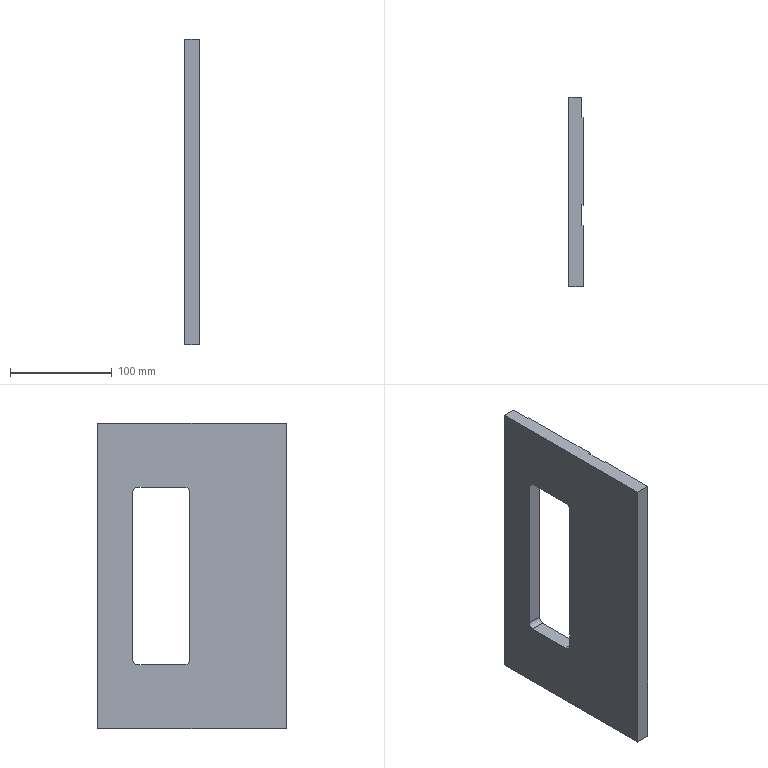Part | SolidWorks | features ICE 3, Extrusion 1, Fillet 1 | 1 solid | 20 faces | box 14 x 185 x 300 mm | volume 622434 mm3 | plane 16 | cylinder 4 | commonest cylinder face diameters 10 x4
STEP:
#1=CARTESIAN_POINT('',(14.,150.5,-82.));
#2=VERTEX_POINT('',#1);
#3=CARTESIAN_POINT('',(14.,150.5,82.));
#4=VERTEX_POINT('',#3);
#5=CARTESIAN_POINT('',(14.,150.5,87.));
#6=DIRECTION('',(0.,0.,1.));
#7=VECTOR('',#6,1000.);
#8=LINE('',#5,#7);
#9=EDGE_CURVE('',#2,#4,#8,.T.);
#10=ORIENTED_EDGE('',*,*,#9,.F.);
#11=CARTESIAN_POINT('',(14.,145.5,-87.));
#12=VERTEX_POINT('',#11);
#13=CARTESIAN_POINT('',(14.,145.5,-82.));
#14=DIRECTION('',(-1.,0.,0.));
#15=DIRECTION('',(0.,-1.,0.));
#16=AXIS2_PLACEMENT_3D('',#13,#14,#15);
#17=CIRCLE('',#16,5.);
#18=EDGE_CURVE('',#2,#12,#17,.T.);
#19=ORIENTED_EDGE('',*,*,#18,.T.);
#20=CARTESIAN_POINT('',(14.,99.5,-87.));
#21=VERTEX_POINT('',#20);
#22=CARTESIAN_POINT('',(14.,94.5,-87.));
#23=DIRECTION('',(0.,1.,0.));
#24=VECTOR('',#23,1000.);
#25=LINE('',#22,#24);
#26=EDGE_CURVE('',#21,#12,#25,.T.);
#27=ORIENTED_EDGE('',*,*,#26,.F.);
#28=CARTESIAN_POINT('',(14.,94.5,-82.));
#29=VERTEX_POINT('',#28);
#30=CARTESIAN_POINT('',(14.,99.5,-82.));
#31=DIRECTION('',(-1.,0.,0.));
#32=DIRECTION('',(0.,-1.,0.));
#33=AXIS2_PLACEMENT_3D('',#30,#31,#32);
#34=CIRCLE('',#33,5.);
#35=EDGE_CURVE('',#21,#29,#34,.T.);
#36=ORIENTED_EDGE('',*,*,#35,.T.);
#37=CARTESIAN_POINT('',(14.,94.5,82.));
#38=VERTEX_POINT('',#37);
#39=CARTESIAN_POINT('',(14.,94.5,87.));
#40=DIRECTION('',(0.,0.,-1.));
#41=VECTOR('',#40,1000.);
#42=LINE('',#39,#41);
#43=EDGE_CURVE('',#38,#29,#42,.T.);
#44=ORIENTED_EDGE('',*,*,#43,.F.);
#45=CARTESIAN_POINT('',(14.,99.5,87.));
#46=VERTEX_POINT('',#45);
#47=CARTESIAN_POINT('',(14.,99.5,82.));
#48=DIRECTION('',(-1.,0.,0.));
#49=DIRECTION('',(0.,-1.,0.));
#50=AXIS2_PLACEMENT_3D('',#47,#48,#49);
#51=CIRCLE('',#50,5.);
#52=EDGE_CURVE('',#38,#46,#51,.T.);
#53=ORIENTED_EDGE('',*,*,#52,.T.);
#54=CARTESIAN_POINT('',(14.,145.5,87.));
#55=VERTEX_POINT('',#54);
#56=CARTESIAN_POINT('',(14.,94.5,87.));
#57=DIRECTION('',(0.,-1.,0.));
#58=VECTOR('',#57,1000.);
#59=LINE('',#56,#58);
#60=EDGE_CURVE('',#55,#46,#59,.T.);
#61=ORIENTED_EDGE('',*,*,#60,.F.);
#62=CARTESIAN_POINT('',(14.,145.5,82.));
#63=DIRECTION('',(-1.,0.,0.));
#64=DIRECTION('',(0.,-1.,0.));
#65=AXIS2_PLACEMENT_3D('',#62,#63,#64);
#66=CIRCLE('',#65,5.);
#67=EDGE_CURVE('',#55,#4,#66,.T.);
#68=ORIENTED_EDGE('',*,*,#67,.T.);
#69=EDGE_LOOP('',(#10,#19,#27,#36,#44,#53,#61,#68));
#70=FACE_BOUND('',#69,.T.);
#71=CARTESIAN_POINT('',(14.,80.,-150.));
#72=VERTEX_POINT('',#71);
#73=CARTESIAN_POINT('',(14.,165.,-150.));
#74=VERTEX_POINT('',#73);
#75=CARTESIAN_POINT('',(14.,185.,-150.));
#76=DIRECTION('',(0.,1.,0.));
#77=VECTOR('',#76,1000.);
#78=LINE('',#75,#77);
#79=EDGE_CURVE('',#72,#74,#78,.T.);
#80=ORIENTED_EDGE('',*,*,#79,.T.);
#81=CARTESIAN_POINT('',(14.,165.,150.));
#82=VERTEX_POINT('',#81);
#83=CARTESIAN_POINT('',(14.,165.,150.));
#84=DIRECTION('',(0.,0.,-1.));
#85=VECTOR('',#84,1000.);
#86=LINE('',#83,#85);
#87=EDGE_CURVE('',#82,#74,#86,.T.);
#88=ORIENTED_EDGE('',*,*,#87,.F.);
#89=CARTESIAN_POINT('',(14.,80.,150.));
#90=VERTEX_POINT('',#89);
#91=CARTESIAN_POINT('',(14.,185.,150.));
#92=DIRECTION('',(0.,1.,0.));
#93=VECTOR('',#92,1000.);
#94=LINE('',#91,#93);
#95=EDGE_CURVE('',#90,#82,#94,.T.);
#96=ORIENTED_EDGE('',*,*,#95,.F.);
#97=CARTESIAN_POINT('',(14.,80.,150.));
#98=DIRECTION('',(0.,0.,1.));
#99=VECTOR('',#98,1000.);
#100=LINE('',#97,#99);
#101=EDGE_CURVE('',#72,#90,#100,.T.);
#102=ORIENTED_EDGE('',*,*,#101,.F.);
#103=EDGE_LOOP('',(#80,#88,#96,#102));
#104=FACE_OUTER_BOUND('',#103,.T.);
#105=CARTESIAN_POINT('',(14.,185.,150.));
#106=DIRECTION('',(-1.,0.,0.));
#107=DIRECTION('',(0.,-1.,0.));
#108=AXIS2_PLACEMENT_3D('',#105,#106,#107);
#109=PLANE('',#108);
#110=ADVANCED_FACE('',(#70,#104),#109,.F.);
#111=CARTESIAN_POINT('',(12.5,185.,-150.));
#112=VERTEX_POINT('',#111);
#113=CARTESIAN_POINT('',(12.5,185.,150.));
#114=VERTEX_POINT('',#113);
#115=CARTESIAN_POINT('',(12.5,185.,150.));
#116=DIRECTION('',(0.,0.,1.));
#117=VECTOR('',#116,1000.);
#118=LINE('',#115,#117);
#119=EDGE_CURVE('',#112,#114,#118,.T.);
#120=ORIENTED_EDGE('',*,*,#119,.F.);
#121=CARTESIAN_POINT('',(0.,185.,-150.));
#122=VERTEX_POINT('',#121);
#123=CARTESIAN_POINT('',(0.,185.,-150.));
#124=DIRECTION('',(-1.,0.,0.));
#125=VECTOR('',#124,1000.);
#126=LINE('',#123,#125);
#127=EDGE_CURVE('',#112,#122,#126,.T.);
#128=ORIENTED_EDGE('',*,*,#127,.T.);
#129=CARTESIAN_POINT('',(0.,185.,150.));
#130=VERTEX_POINT('',#129);
#131=CARTESIAN_POINT('',(0.,185.,150.));
#132=DIRECTION('',(0.,0.,-1.));
#133=VECTOR('',#132,1000.);
#134=LINE('',#131,#133);
#135=EDGE_CURVE('',#130,#122,#134,.T.);
#136=ORIENTED_EDGE('',*,*,#135,.F.);
#137=CARTESIAN_POINT('',(0.,185.,150.));
#138=DIRECTION('',(-1.,0.,0.));
#139=VECTOR('',#138,1000.);
#140=LINE('',#137,#139);
#141=EDGE_CURVE('',#114,#130,#140,.T.);
#142=ORIENTED_EDGE('',*,*,#141,.F.);
#143=EDGE_LOOP('',(#120,#128,#136,#142));
#144=FACE_OUTER_BOUND('',#143,.T.);
#145=CARTESIAN_POINT('',(0.,185.,150.));
#146=DIRECTION('',(0.,-1.,0.));
#147=DIRECTION('',(0.,0.,-1.));
#148=AXIS2_PLACEMENT_3D('',#145,#146,#147);
#149=PLANE('',#148);
#150=ADVANCED_FACE('',(#144),#149,.F.);
#151=CARTESIAN_POINT('',(0.,0.,-150.));
#152=VERTEX_POINT('',#151);
#153=CARTESIAN_POINT('',(14.,0.,-150.));
#154=VERTEX_POINT('',#153);
#155=CARTESIAN_POINT('',(0.,0.,-150.));
#156=DIRECTION('',(1.,0.,0.));
#157=VECTOR('',#156,1000.);
#158=LINE('',#155,#157);
#159=EDGE_CURVE('',#152,#154,#158,.T.);
#160=ORIENTED_EDGE('',*,*,#159,.T.);
#161=CARTESIAN_POINT('',(14.,0.,150.));
#162=VERTEX_POINT('',#161);
#163=CARTESIAN_POINT('',(14.,0.,150.));
#164=DIRECTION('',(0.,0.,-1.));
#165=VECTOR('',#164,1000.);
#166=LINE('',#163,#165);
#167=EDGE_CURVE('',#162,#154,#166,.T.);
#168=ORIENTED_EDGE('',*,*,#167,.F.);
#169=CARTESIAN_POINT('',(0.,0.,150.));
#170=VERTEX_POINT('',#169);
#171=CARTESIAN_POINT('',(0.,0.,150.));
#172=DIRECTION('',(1.,0.,0.));
#173=VECTOR('',#172,1000.);
#174=LINE('',#171,#173);
#175=EDGE_CURVE('',#170,#162,#174,.T.);
#176=ORIENTED_EDGE('',*,*,#175,.F.);
#177=CARTESIAN_POINT('',(0.,0.,150.));
#178=DIRECTION('',(0.,0.,-1.));
#179=VECTOR('',#178,1000.);
#180=LINE('',#177,#179);
#181=EDGE_CURVE('',#170,#152,#180,.T.);
#182=ORIENTED_EDGE('',*,*,#181,.T.);
#183=EDGE_LOOP('',(#160,#168,#176,#182));
#184=FACE_OUTER_BOUND('',#183,.T.);
#185=CARTESIAN_POINT('',(0.,0.,150.));
#186=DIRECTION('',(0.,1.,0.));
#187=DIRECTION('',(0.,0.,1.));
#188=AXIS2_PLACEMENT_3D('',#185,#186,#187);
#189=PLANE('',#188);
#190=ADVANCED_FACE('',(#184),#189,.F.);
#191=CARTESIAN_POINT('',(14.,59.,-150.));
#192=VERTEX_POINT('',#191);
#193=CARTESIAN_POINT('',(14.,185.,-150.));
#194=DIRECTION('',(0.,1.,0.));
#195=VECTOR('',#194,1000.);
#196=LINE('',#193,#195);
#197=EDGE_CURVE('',#154,#192,#196,.T.);
#198=ORIENTED_EDGE('',*,*,#197,.T.);
#199=CARTESIAN_POINT('',(14.,59.,150.));
#200=VERTEX_POINT('',#199);
#201=CARTESIAN_POINT('',(14.,59.,150.));
#202=DIRECTION('',(0.,0.,-1.));
#203=VECTOR('',#202,1000.);
#204=LINE('',#201,#203);
#205=EDGE_CURVE('',#200,#192,#204,.T.);
#206=ORIENTED_EDGE('',*,*,#205,.F.);
#207=CARTESIAN_POINT('',(14.,185.,150.));
#208=DIRECTION('',(0.,1.,0.));
#209=VECTOR('',#208,1000.);
#210=LINE('',#207,#209);
#211=EDGE_CURVE('',#162,#200,#210,.T.);
#212=ORIENTED_EDGE('',*,*,#211,.F.);
#213=ORIENTED_EDGE('',*,*,#167,.T.);
#214=EDGE_LOOP('',(#198,#206,#212,#213));
#215=FACE_OUTER_BOUND('',#214,.T.);
#216=CARTESIAN_POINT('',(14.,185.,150.));
#217=DIRECTION('',(-1.,0.,0.));
#218=DIRECTION('',(0.,-1.,0.));
#219=AXIS2_PLACEMENT_3D('',#216,#217,#218);
#220=PLANE('',#219);
#221=ADVANCED_FACE('',(#215),#220,.F.);
#222=CARTESIAN_POINT('',(0.,94.5,-82.));
#223=VERTEX_POINT('',#222);
#224=CARTESIAN_POINT('',(0.,94.5,82.));
#225=VERTEX_POINT('',#224);
#226=CARTESIAN_POINT('',(0.,94.5,87.));
#227=DIRECTION('',(0.,0.,1.));
#228=VECTOR('',#227,1000.);
#229=LINE('',#226,#228);
#230=EDGE_CURVE('',#223,#225,#229,.T.);
#231=ORIENTED_EDGE('',*,*,#230,.F.);
#232=CARTESIAN_POINT('',(0.,99.5,-87.));
#233=VERTEX_POINT('',#232);
#234=CARTESIAN_POINT('',(0.,99.5,-82.));
#235=DIRECTION('',(1.,0.,0.));
#236=DIRECTION('',(0.,1.,0.));
#237=AXIS2_PLACEMENT_3D('',#234,#235,#236);
#238=CIRCLE('',#237,5.);
#239=EDGE_CURVE('',#223,#233,#238,.T.);
#240=ORIENTED_EDGE('',*,*,#239,.T.);
#241=CARTESIAN_POINT('',(0.,145.5,-87.));
#242=VERTEX_POINT('',#241);
#243=CARTESIAN_POINT('',(0.,94.5,-87.));
#244=DIRECTION('',(0.,-1.,0.));
#245=VECTOR('',#244,1000.);
#246=LINE('',#243,#245);
#247=EDGE_CURVE('',#242,#233,#246,.T.);
#248=ORIENTED_EDGE('',*,*,#247,.F.);
#249=CARTESIAN_POINT('',(0.,150.5,-82.));
#250=VERTEX_POINT('',#249);
#251=CARTESIAN_POINT('',(0.,145.5,-82.));
#252=DIRECTION('',(1.,0.,0.));
#253=DIRECTION('',(0.,1.,0.));
#254=AXIS2_PLACEMENT_3D('',#251,#252,#253);
#255=CIRCLE('',#254,5.);
#256=EDGE_CURVE('',#242,#250,#255,.T.);
#257=ORIENTED_EDGE('',*,*,#256,.T.);
#258=CARTESIAN_POINT('',(0.,150.5,82.));
#259=VERTEX_POINT('',#258);
#260=CARTESIAN_POINT('',(0.,150.5,87.));
#261=DIRECTION('',(0.,0.,-1.));
#262=VECTOR('',#261,1000.);
#263=LINE('',#260,#262);
#264=EDGE_CURVE('',#259,#250,#263,.T.);
#265=ORIENTED_EDGE('',*,*,#264,.F.);
#266=CARTESIAN_POINT('',(0.,145.5,87.));
#267=VERTEX_POINT('',#266);
#268=CARTESIAN_POINT('',(0.,145.5,82.));
#269=DIRECTION('',(1.,0.,0.));
#270=DIRECTION('',(0.,1.,0.));
#271=AXIS2_PLACEMENT_3D('',#268,#269,#270);
#272=CIRCLE('',#271,5.);
#273=EDGE_CURVE('',#259,#267,#272,.T.);
#274=ORIENTED_EDGE('',*,*,#273,.T.);
#275=CARTESIAN_POINT('',(0.,99.5,87.));
#276=VERTEX_POINT('',#275);
#277=CARTESIAN_POINT('',(0.,94.5,87.));
#278=DIRECTION('',(0.,1.,0.));
#279=VECTOR('',#278,1000.);
#280=LINE('',#277,#279);
#281=EDGE_CURVE('',#276,#267,#280,.T.);
#282=ORIENTED_EDGE('',*,*,#281,.F.);
#283=CARTESIAN_POINT('',(0.,99.5,82.));
#284=DIRECTION('',(1.,0.,0.));
#285=DIRECTION('',(0.,1.,0.));
#286=AXIS2_PLACEMENT_3D('',#283,#284,#285);
#287=CIRCLE('',#286,5.);
#288=EDGE_CURVE('',#276,#225,#287,.T.);
#289=ORIENTED_EDGE('',*,*,#288,.T.);
#290=EDGE_LOOP('',(#231,#240,#248,#257,#265,#274,#282,#289));
#291=FACE_BOUND('',#290,.T.);
#292=CARTESIAN_POINT('',(0.,0.,-150.));
#293=DIRECTION('',(0.,-1.,0.));
#294=VECTOR('',#293,1000.);
#295=LINE('',#292,#294);
#296=EDGE_CURVE('',#122,#152,#295,.T.);
#297=ORIENTED_EDGE('',*,*,#296,.T.);
#298=ORIENTED_EDGE('',*,*,#181,.F.);
#299=CARTESIAN_POINT('',(0.,0.,150.));
#300=DIRECTION('',(0.,-1.,0.));
#301=VECTOR('',#300,1000.);
#302=LINE('',#299,#301);
#303=EDGE_CURVE('',#130,#170,#302,.T.);
#304=ORIENTED_EDGE('',*,*,#303,.F.);
#305=ORIENTED_EDGE('',*,*,#135,.T.);
#306=EDGE_LOOP('',(#297,#298,#304,#305));
#307=FACE_OUTER_BOUND('',#306,.T.);
#308=CARTESIAN_POINT('',(0.,0.,150.));
#309=DIRECTION('',(1.,0.,0.));
#310=DIRECTION('',(0.,1.,0.));
#311=AXIS2_PLACEMENT_3D('',#308,#309,#310);
#312=PLANE('',#311);
#313=ADVANCED_FACE('',(#291,#307),#312,.F.);
#314=ORIENTED_EDGE('',*,*,#95,.T.);
#315=CARTESIAN_POINT('',(12.5,165.,150.));
#316=VERTEX_POINT('',#315);
#317=CARTESIAN_POINT('',(12.5,165.,150.));
#318=DIRECTION('',(1.,0.,0.));
#319=VECTOR('',#318,1000.);
#320=LINE('',#317,#319);
#321=EDGE_CURVE('',#316,#82,#320,.T.);
#322=ORIENTED_EDGE('',*,*,#321,.F.);
#323=CARTESIAN_POINT('',(12.5,185.,150.));
#324=DIRECTION('',(0.,-1.,0.));
#325=VECTOR('',#324,1000.);
#326=LINE('',#323,#325);
#327=EDGE_CURVE('',#114,#316,#326,.T.);
#328=ORIENTED_EDGE('',*,*,#327,.F.);
#329=ORIENTED_EDGE('',*,*,#141,.T.);
#330=ORIENTED_EDGE('',*,*,#303,.T.);
#331=ORIENTED_EDGE('',*,*,#175,.T.);
#332=ORIENTED_EDGE('',*,*,#211,.T.);
#333=CARTESIAN_POINT('',(12.5,59.,150.));
#334=VERTEX_POINT('',#333);
#335=CARTESIAN_POINT('',(12.5,59.,150.));
#336=DIRECTION('',(1.,0.,0.));
#337=VECTOR('',#336,1000.);
#338=LINE('',#335,#337);
#339=EDGE_CURVE('',#334,#200,#338,.T.);
#340=ORIENTED_EDGE('',*,*,#339,.F.);
#341=CARTESIAN_POINT('',(12.5,80.,150.));
#342=VERTEX_POINT('',#341);
#343=CARTESIAN_POINT('',(12.5,80.,150.));
#344=DIRECTION('',(0.,-1.,0.));
#345=VECTOR('',#344,1000.);
#346=LINE('',#343,#345);
#347=EDGE_CURVE('',#342,#334,#346,.T.);
#348=ORIENTED_EDGE('',*,*,#347,.F.);
#349=CARTESIAN_POINT('',(12.5,80.,150.));
#350=DIRECTION('',(1.,0.,0.));
#351=VECTOR('',#350,1000.);
#352=LINE('',#349,#351);
#353=EDGE_CURVE('',#342,#90,#352,.T.);
#354=ORIENTED_EDGE('',*,*,#353,.T.);
#355=EDGE_LOOP('',(#314,#322,#328,#329,#330,#331,#332,#340,#348,#354));
#356=FACE_OUTER_BOUND('',#355,.T.);
#357=CARTESIAN_POINT('',(0.,0.,150.));
#358=DIRECTION('',(0.,0.,-1.));
#359=DIRECTION('',(-1.,0.,0.));
#360=AXIS2_PLACEMENT_3D('',#357,#358,#359);
#361=PLANE('',#360);
#362=ADVANCED_FACE('',(#356),#361,.F.);
#363=CARTESIAN_POINT('',(12.5,165.,-150.));
#364=VERTEX_POINT('',#363);
#365=CARTESIAN_POINT('',(12.5,165.,-150.));
#366=DIRECTION('',(1.,0.,0.));
#367=VECTOR('',#366,1000.);
#368=LINE('',#365,#367);
#369=EDGE_CURVE('',#364,#74,#368,.T.);
#370=ORIENTED_EDGE('',*,*,#369,.T.);
#371=ORIENTED_EDGE('',*,*,#79,.F.);
#372=CARTESIAN_POINT('',(12.5,80.,-150.));
#373=VERTEX_POINT('',#372);
#374=CARTESIAN_POINT('',(12.5,80.,-150.));
#375=DIRECTION('',(1.,0.,0.));
#376=VECTOR('',#375,1000.);
#377=LINE('',#374,#376);
#378=EDGE_CURVE('',#373,#72,#377,.T.);
#379=ORIENTED_EDGE('',*,*,#378,.F.);
#380=CARTESIAN_POINT('',(12.5,59.,-150.));
#381=VERTEX_POINT('',#380);
#382=CARTESIAN_POINT('',(12.5,80.,-150.));
#383=DIRECTION('',(0.,1.,0.));
#384=VECTOR('',#383,1000.);
#385=LINE('',#382,#384);
#386=EDGE_CURVE('',#381,#373,#385,.T.);
#387=ORIENTED_EDGE('',*,*,#386,.F.);
#388=CARTESIAN_POINT('',(12.5,59.,-150.));
#389=DIRECTION('',(1.,0.,0.));
#390=VECTOR('',#389,1000.);
#391=LINE('',#388,#390);
#392=EDGE_CURVE('',#381,#192,#391,.T.);
#393=ORIENTED_EDGE('',*,*,#392,.T.);
#394=ORIENTED_EDGE('',*,*,#197,.F.);
#395=ORIENTED_EDGE('',*,*,#159,.F.);
#396=ORIENTED_EDGE('',*,*,#296,.F.);
#397=ORIENTED_EDGE('',*,*,#127,.F.);
#398=CARTESIAN_POINT('',(12.5,185.,-150.));
#399=DIRECTION('',(0.,1.,0.));
#400=VECTOR('',#399,1000.);
#401=LINE('',#398,#400);
#402=EDGE_CURVE('',#364,#112,#401,.T.);
#403=ORIENTED_EDGE('',*,*,#402,.F.);
#404=EDGE_LOOP('',(#370,#371,#379,#387,#393,#394,#395,#396,#397,#403));
#405=FACE_OUTER_BOUND('',#404,.T.);
#406=CARTESIAN_POINT('',(0.,0.,-150.));
#407=DIRECTION('',(0.,0.,-1.));
#408=DIRECTION('',(-1.,0.,0.));
#409=AXIS2_PLACEMENT_3D('',#406,#407,#408);
#410=PLANE('',#409);
#411=ADVANCED_FACE('',(#405),#410,.T.);
#412=ORIENTED_EDGE('',*,*,#101,.T.);
#413=ORIENTED_EDGE('',*,*,#353,.F.);
#414=CARTESIAN_POINT('',(12.5,80.,150.));
#415=DIRECTION('',(0.,0.,1.));
#416=VECTOR('',#415,1000.);
#417=LINE('',#414,#416);
#418=EDGE_CURVE('',#373,#342,#417,.T.);
#419=ORIENTED_EDGE('',*,*,#418,.F.);
#420=ORIENTED_EDGE('',*,*,#378,.T.);
#421=EDGE_LOOP('',(#412,#413,#419,#420));
#422=FACE_OUTER_BOUND('',#421,.T.);
#423=CARTESIAN_POINT('',(12.5,80.,150.));
#424=DIRECTION('',(0.,1.,0.));
#425=DIRECTION('',(-1.,0.,0.));
#426=AXIS2_PLACEMENT_3D('',#423,#424,#425);
#427=PLANE('',#426);
#428=ADVANCED_FACE('',(#422),#427,.F.);
#429=ORIENTED_EDGE('',*,*,#205,.T.);
#430=ORIENTED_EDGE('',*,*,#392,.F.);
#431=CARTESIAN_POINT('',(12.5,59.,150.));
#432=DIRECTION('',(0.,0.,-1.));
#433=VECTOR('',#432,1000.);
#434=LINE('',#431,#433);
#435=EDGE_CURVE('',#334,#381,#434,.T.);
#436=ORIENTED_EDGE('',*,*,#435,.F.);
#437=ORIENTED_EDGE('',*,*,#339,.T.);
#438=EDGE_LOOP('',(#429,#430,#436,#437));
#439=FACE_OUTER_BOUND('',#438,.T.);
#440=CARTESIAN_POINT('',(12.5,59.,150.));
#441=DIRECTION('',(0.,-1.,0.));
#442=DIRECTION('',(1.,0.,0.));
#443=AXIS2_PLACEMENT_3D('',#440,#441,#442);
#444=PLANE('',#443);
#445=ADVANCED_FACE('',(#439),#444,.F.);
#446=ORIENTED_EDGE('',*,*,#347,.T.);
#447=ORIENTED_EDGE('',*,*,#435,.T.);
#448=ORIENTED_EDGE('',*,*,#386,.T.);
#449=ORIENTED_EDGE('',*,*,#418,.T.);
#450=EDGE_LOOP('',(#446,#447,#448,#449));
#451=FACE_OUTER_BOUND('',#450,.T.);
#452=CARTESIAN_POINT('',(12.5,0.,0.));
#453=DIRECTION('',(1.,0.,0.));
#454=DIRECTION('',(0.,1.,0.));
#455=AXIS2_PLACEMENT_3D('',#452,#453,#454);
#456=PLANE('',#455);
#457=ADVANCED_FACE('',(#451),#456,.T.);
#458=ORIENTED_EDGE('',*,*,#87,.T.);
#459=ORIENTED_EDGE('',*,*,#369,.F.);
#460=CARTESIAN_POINT('',(12.5,165.,150.));
#461=DIRECTION('',(0.,0.,-1.));
#462=VECTOR('',#461,1000.);
#463=LINE('',#460,#462);
#464=EDGE_CURVE('',#316,#364,#463,.T.);
#465=ORIENTED_EDGE('',*,*,#464,.F.);
#466=ORIENTED_EDGE('',*,*,#321,.T.);
#467=EDGE_LOOP('',(#458,#459,#465,#466));
#468=FACE_OUTER_BOUND('',#467,.T.);
#469=CARTESIAN_POINT('',(12.5,165.,150.));
#470=DIRECTION('',(0.,-1.,0.));
#471=DIRECTION('',(1.,0.,0.));
#472=AXIS2_PLACEMENT_3D('',#469,#470,#471);
#473=PLANE('',#472);
#474=ADVANCED_FACE('',(#468),#473,.F.);
#475=ORIENTED_EDGE('',*,*,#327,.T.);
#476=ORIENTED_EDGE('',*,*,#464,.T.);
#477=ORIENTED_EDGE('',*,*,#402,.T.);
#478=ORIENTED_EDGE('',*,*,#119,.T.);
#479=EDGE_LOOP('',(#475,#476,#477,#478));
#480=FACE_OUTER_BOUND('',#479,.T.);
#481=CARTESIAN_POINT('',(12.5,0.,0.));
#482=DIRECTION('',(1.,0.,0.));
#483=DIRECTION('',(0.,1.,0.));
#484=AXIS2_PLACEMENT_3D('',#481,#482,#483);
#485=PLANE('',#484);
#486=ADVANCED_FACE('',(#480),#485,.T.);
#487=ORIENTED_EDGE('',*,*,#247,.T.);
#488=CARTESIAN_POINT('',(14.,99.5,-87.));
#489=DIRECTION('',(1.,0.,0.));
#490=VECTOR('',#489,1000.);
#491=LINE('',#488,#490);
#492=EDGE_CURVE('',#233,#21,#491,.T.);
#493=ORIENTED_EDGE('',*,*,#492,.T.);
#494=ORIENTED_EDGE('',*,*,#26,.T.);
#495=CARTESIAN_POINT('',(0.,145.5,-87.));
#496=DIRECTION('',(-1.,0.,0.));
#497=VECTOR('',#496,1000.);
#498=LINE('',#495,#497);
#499=EDGE_CURVE('',#12,#242,#498,.T.);
#500=ORIENTED_EDGE('',*,*,#499,.T.);
#501=EDGE_LOOP('',(#487,#493,#494,#500));
#502=FACE_OUTER_BOUND('',#501,.T.);
#503=CARTESIAN_POINT('',(-0.001,94.5,-87.));
#504=DIRECTION('',(0.,0.,-1.));
#505=DIRECTION('',(-1.,0.,0.));
#506=AXIS2_PLACEMENT_3D('',#503,#504,#505);
#507=PLANE('',#506);
#508=ADVANCED_FACE('',(#502),#507,.F.);
#509=ORIENTED_EDGE('',*,*,#230,.T.);
#510=CARTESIAN_POINT('',(14.,94.5,82.));
#511=DIRECTION('',(1.,0.,0.));
#512=VECTOR('',#511,1000.);
#513=LINE('',#510,#512);
#514=EDGE_CURVE('',#225,#38,#513,.T.);
#515=ORIENTED_EDGE('',*,*,#514,.T.);
#516=ORIENTED_EDGE('',*,*,#43,.T.);
#517=CARTESIAN_POINT('',(0.,94.5,-82.));
#518=DIRECTION('',(-1.,0.,0.));
#519=VECTOR('',#518,1000.);
#520=LINE('',#517,#519);
#521=EDGE_CURVE('',#29,#223,#520,.T.);
#522=ORIENTED_EDGE('',*,*,#521,.T.);
#523=EDGE_LOOP('',(#509,#515,#516,#522));
#524=FACE_OUTER_BOUND('',#523,.T.);
#525=CARTESIAN_POINT('',(-0.001,94.5,87.));
#526=DIRECTION('',(0.,-1.,0.));
#527=DIRECTION('',(1.,0.,0.));
#528=AXIS2_PLACEMENT_3D('',#525,#526,#527);
#529=PLANE('',#528);
#530=ADVANCED_FACE('',(#524),#529,.F.);
#531=ORIENTED_EDGE('',*,*,#60,.T.);
#532=CARTESIAN_POINT('',(0.,99.5,87.));
#533=DIRECTION('',(-1.,0.,0.));
#534=VECTOR('',#533,1000.);
#535=LINE('',#532,#534);
#536=EDGE_CURVE('',#46,#276,#535,.T.);
#537=ORIENTED_EDGE('',*,*,#536,.T.);
#538=ORIENTED_EDGE('',*,*,#281,.T.);
#539=CARTESIAN_POINT('',(14.,145.5,87.));
#540=DIRECTION('',(1.,0.,0.));
#541=VECTOR('',#540,1000.);
#542=LINE('',#539,#541);
#543=EDGE_CURVE('',#267,#55,#542,.T.);
#544=ORIENTED_EDGE('',*,*,#543,.T.);
#545=EDGE_LOOP('',(#531,#537,#538,#544));
#546=FACE_OUTER_BOUND('',#545,.T.);
#547=CARTESIAN_POINT('',(-0.001,94.5,87.));
#548=DIRECTION('',(0.,0.,1.));
#549=DIRECTION('',(1.,0.,0.));
#550=AXIS2_PLACEMENT_3D('',#547,#548,#549);
#551=PLANE('',#550);
#552=ADVANCED_FACE('',(#546),#551,.F.);
#553=ORIENTED_EDGE('',*,*,#9,.T.);
#554=CARTESIAN_POINT('',(0.,150.5,82.));
#555=DIRECTION('',(-1.,0.,0.));
#556=VECTOR('',#555,1000.);
#557=LINE('',#554,#556);
#558=EDGE_CURVE('',#4,#259,#557,.T.);
#559=ORIENTED_EDGE('',*,*,#558,.T.);
#560=ORIENTED_EDGE('',*,*,#264,.T.);
#561=CARTESIAN_POINT('',(14.,150.5,-82.));
#562=DIRECTION('',(1.,0.,0.));
#563=VECTOR('',#562,1000.);
#564=LINE('',#561,#563);
#565=EDGE_CURVE('',#250,#2,#564,.T.);
#566=ORIENTED_EDGE('',*,*,#565,.T.);
#567=EDGE_LOOP('',(#553,#559,#560,#566));
#568=FACE_OUTER_BOUND('',#567,.T.);
#569=CARTESIAN_POINT('',(-0.001,150.5,87.));
#570=DIRECTION('',(0.,1.,0.));
#571=DIRECTION('',(-1.,0.,0.));
#572=AXIS2_PLACEMENT_3D('',#569,#570,#571);
#573=PLANE('',#572);
#574=ADVANCED_FACE('',(#568),#573,.F.);
#575=ORIENTED_EDGE('',*,*,#288,.F.);
#576=ORIENTED_EDGE('',*,*,#536,.F.);
#577=ORIENTED_EDGE('',*,*,#52,.F.);
#578=ORIENTED_EDGE('',*,*,#514,.F.);
#579=EDGE_LOOP('',(#575,#576,#577,#578));
#580=FACE_OUTER_BOUND('',#579,.T.);
#581=CARTESIAN_POINT('',(-0.001,99.5,82.));
#582=DIRECTION('',(-1.,0.,0.));
#583=DIRECTION('',(0.,-1.,0.));
#584=AXIS2_PLACEMENT_3D('',#581,#582,#583);
#585=CYLINDRICAL_SURFACE('',#584,5.);
#586=ADVANCED_FACE('',(#580),#585,.F.);
#587=ORIENTED_EDGE('',*,*,#273,.F.);
#588=ORIENTED_EDGE('',*,*,#558,.F.);
#589=ORIENTED_EDGE('',*,*,#67,.F.);
#590=ORIENTED_EDGE('',*,*,#543,.F.);
#591=EDGE_LOOP('',(#587,#588,#589,#590));
#592=FACE_OUTER_BOUND('',#591,.T.);
#593=CARTESIAN_POINT('',(-0.001,145.5,82.));
#594=DIRECTION('',(-1.,0.,0.));
#595=DIRECTION('',(0.,-1.,0.));
#596=AXIS2_PLACEMENT_3D('',#593,#594,#595);
#597=CYLINDRICAL_SURFACE('',#596,5.);
#598=ADVANCED_FACE('',(#592),#597,.F.);
#599=ORIENTED_EDGE('',*,*,#239,.F.);
#600=ORIENTED_EDGE('',*,*,#521,.F.);
#601=ORIENTED_EDGE('',*,*,#35,.F.);
#602=ORIENTED_EDGE('',*,*,#492,.F.);
#603=EDGE_LOOP('',(#599,#600,#601,#602));
#604=FACE_OUTER_BOUND('',#603,.T.);
#605=CARTESIAN_POINT('',(-0.001,99.5,-82.));
#606=DIRECTION('',(-1.,0.,0.));
#607=DIRECTION('',(0.,-1.,0.));
#608=AXIS2_PLACEMENT_3D('',#605,#606,#607);
#609=CYLINDRICAL_SURFACE('',#608,5.);
#610=ADVANCED_FACE('',(#604),#609,.F.);
#611=ORIENTED_EDGE('',*,*,#256,.F.);
#612=ORIENTED_EDGE('',*,*,#499,.F.);
#613=ORIENTED_EDGE('',*,*,#18,.F.);
#614=ORIENTED_EDGE('',*,*,#565,.F.);
#615=EDGE_LOOP('',(#611,#612,#613,#614));
#616=FACE_OUTER_BOUND('',#615,.T.);
#617=CARTESIAN_POINT('',(-0.001,145.5,-82.));
#618=DIRECTION('',(-1.,0.,0.));
#619=DIRECTION('',(0.,-1.,0.));
#620=AXIS2_PLACEMENT_3D('',#617,#618,#619);
#621=CYLINDRICAL_SURFACE('',#620,5.);
#622=ADVANCED_FACE('',(#616),#621,.F.);
#623=CLOSED_SHELL('',(#110,#150,#190,#221,#313,#362,#411,#428,#445,#457,#474,#486,#508,#530,#552,#574,#586,#598,#610,#622));
#624=MANIFOLD_SOLID_BREP('',#623);
#625=CARTESIAN_POINT('',(0.,0.,0.));
#626=DIRECTION('',(0.,0.,1.));
#627=DIRECTION('',(1.,0.,0.));
#628=AXIS2_PLACEMENT_3D('',#625,#626,#627);
#629=(LENGTH_UNIT()NAMED_UNIT(*)SI_UNIT(.MILLI.,.METRE.));
#630=UNCERTAINTY_MEASURE_WITH_UNIT(LENGTH_MEASURE(0.00001),#629,'','');
#631=(NAMED_UNIT(*)PLANE_ANGLE_UNIT()SI_UNIT($,.RADIAN.));
#632=(NAMED_UNIT(*)SI_UNIT($,.STERADIAN.)SOLID_ANGLE_UNIT());
#633=(GEOMETRIC_REPRESENTATION_CONTEXT(3)GLOBAL_UNCERTAINTY_ASSIGNED_CONTEXT((#630))GLOBAL_UNIT_ASSIGNED_CONTEXT((#629,#631,#632))REPRESENTATION_CONTEXT('',''));
#634=ADVANCED_BREP_SHAPE_REPRESENTATION('',(#624,#628),#633);